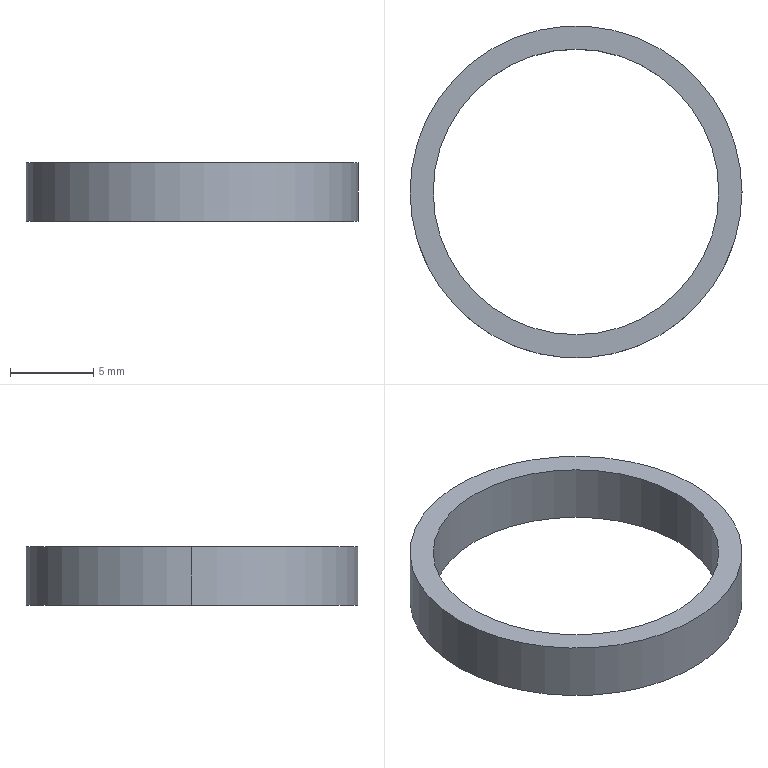Part | NX | features BREP 1 | 1 solid | 6 faces | box 20 x 20 x 3.5 mm | volume 286.325 mm3 | cylinder 4 | plane 2 | commonest cylinder face diameters 17.2 x2 20 x2
STEP:
#1=CARTESIAN_POINT('',(-8.6,0.,0.));
#2=VERTEX_POINT('',#1);
#3=CARTESIAN_POINT('',(8.6,0.,0.));
#4=VERTEX_POINT('',#3);
#5=CARTESIAN_POINT('',(0.,0.,0.));
#6=DIRECTION('',(0.,0.,1.));
#7=DIRECTION('',(1.,0.,0.));
#8=AXIS2_PLACEMENT_3D('',#5,#6,#7);
#9=CIRCLE('',#8,8.6);
#10=EDGE_CURVE('',#2,#4,#9,.T.);
#11=ORIENTED_EDGE('',*,*,#10,.F.);
#12=CARTESIAN_POINT('',(-8.6,0.,3.5));
#13=VERTEX_POINT('',#12);
#14=CARTESIAN_POINT('',(-8.6,0.,0.));
#15=DIRECTION('',(0.,0.,1.));
#16=VECTOR('',#15,1000.);
#17=LINE('',#14,#16);
#18=EDGE_CURVE('',#13,#2,#17,.F.);
#19=ORIENTED_EDGE('',*,*,#18,.F.);
#20=CARTESIAN_POINT('',(8.6,0.,3.5));
#21=VERTEX_POINT('',#20);
#22=CARTESIAN_POINT('',(0.,0.,3.5));
#23=DIRECTION('',(0.,0.,1.));
#24=DIRECTION('',(1.,0.,0.));
#25=AXIS2_PLACEMENT_3D('',#22,#23,#24);
#26=CIRCLE('',#25,8.6);
#27=EDGE_CURVE('',#13,#21,#26,.T.);
#28=ORIENTED_EDGE('',*,*,#27,.T.);
#29=CARTESIAN_POINT('',(8.6,0.,0.));
#30=DIRECTION('',(0.,0.,1.));
#31=VECTOR('',#30,1000.);
#32=LINE('',#29,#31);
#33=EDGE_CURVE('',#21,#4,#32,.F.);
#34=ORIENTED_EDGE('',*,*,#33,.T.);
#35=EDGE_LOOP('',(#11,#19,#28,#34));
#36=FACE_BOUND('',#35,.T.);
#37=CARTESIAN_POINT('',(0.,0.,0.));
#38=DIRECTION('',(0.,0.,1.));
#39=DIRECTION('',(1.,0.,0.));
#40=AXIS2_PLACEMENT_3D('',#37,#38,#39);
#41=CYLINDRICAL_SURFACE('',#40,8.6);
#42=ADVANCED_FACE('',(#36),#41,.F.);
#43=CARTESIAN_POINT('',(10.,0.,3.5));
#44=VERTEX_POINT('',#43);
#45=CARTESIAN_POINT('',(-10.,0.,3.5));
#46=VERTEX_POINT('',#45);
#47=CARTESIAN_POINT('',(0.,0.,3.5));
#48=DIRECTION('',(0.,0.,1.));
#49=DIRECTION('',(1.,0.,0.));
#50=AXIS2_PLACEMENT_3D('',#47,#48,#49);
#51=CIRCLE('',#50,10.);
#52=EDGE_CURVE('',#44,#46,#51,.T.);
#53=ORIENTED_EDGE('',*,*,#52,.F.);
#54=CARTESIAN_POINT('',(10.,0.,0.));
#55=VERTEX_POINT('',#54);
#56=CARTESIAN_POINT('',(10.,0.,3.5));
#57=DIRECTION('',(0.,0.,-1.));
#58=VECTOR('',#57,1000.);
#59=LINE('',#56,#58);
#60=EDGE_CURVE('',#44,#55,#59,.T.);
#61=ORIENTED_EDGE('',*,*,#60,.T.);
#62=CARTESIAN_POINT('',(-10.,0.,0.));
#63=VERTEX_POINT('',#62);
#64=CARTESIAN_POINT('',(0.,0.,0.));
#65=DIRECTION('',(0.,0.,1.));
#66=DIRECTION('',(1.,0.,0.));
#67=AXIS2_PLACEMENT_3D('',#64,#65,#66);
#68=CIRCLE('',#67,10.);
#69=EDGE_CURVE('',#55,#63,#68,.T.);
#70=ORIENTED_EDGE('',*,*,#69,.T.);
#71=CARTESIAN_POINT('',(-10.,0.,3.5));
#72=DIRECTION('',(0.,0.,-1.));
#73=VECTOR('',#72,1000.);
#74=LINE('',#71,#73);
#75=EDGE_CURVE('',#46,#63,#74,.T.);
#76=ORIENTED_EDGE('',*,*,#75,.F.);
#77=EDGE_LOOP('',(#53,#61,#70,#76));
#78=FACE_BOUND('',#77,.T.);
#79=CARTESIAN_POINT('',(0.,0.,3.5));
#80=DIRECTION('',(0.,0.,-1.));
#81=DIRECTION('',(-1.,0.,0.));
#82=AXIS2_PLACEMENT_3D('',#79,#80,#81);
#83=CYLINDRICAL_SURFACE('',#82,10.);
#84=ADVANCED_FACE('',(#78),#83,.T.);
#85=ORIENTED_EDGE('',*,*,#60,.F.);
#86=CARTESIAN_POINT('',(0.,0.,3.5));
#87=DIRECTION('',(0.,0.,1.));
#88=DIRECTION('',(1.,0.,0.));
#89=AXIS2_PLACEMENT_3D('',#86,#87,#88);
#90=CIRCLE('',#89,10.);
#91=EDGE_CURVE('',#46,#44,#90,.T.);
#92=ORIENTED_EDGE('',*,*,#91,.F.);
#93=ORIENTED_EDGE('',*,*,#75,.T.);
#94=CARTESIAN_POINT('',(0.,0.,0.));
#95=DIRECTION('',(0.,0.,1.));
#96=DIRECTION('',(1.,0.,0.));
#97=AXIS2_PLACEMENT_3D('',#94,#95,#96);
#98=CIRCLE('',#97,10.);
#99=EDGE_CURVE('',#63,#55,#98,.T.);
#100=ORIENTED_EDGE('',*,*,#99,.T.);
#101=EDGE_LOOP('',(#85,#92,#93,#100));
#102=FACE_BOUND('',#101,.T.);
#103=CARTESIAN_POINT('',(0.,0.,3.5));
#104=DIRECTION('',(0.,0.,-1.));
#105=DIRECTION('',(-1.,0.,0.));
#106=AXIS2_PLACEMENT_3D('',#103,#104,#105);
#107=CYLINDRICAL_SURFACE('',#106,10.);
#108=ADVANCED_FACE('',(#102),#107,.T.);
#109=ORIENTED_EDGE('',*,*,#91,.T.);
#110=ORIENTED_EDGE('',*,*,#52,.T.);
#111=EDGE_LOOP('',(#109,#110));
#112=FACE_BOUND('',#111,.T.);
#113=CARTESIAN_POINT('',(0.,0.,3.5));
#114=DIRECTION('',(0.,0.,1.));
#115=DIRECTION('',(1.,0.,0.));
#116=AXIS2_PLACEMENT_3D('',#113,#114,#115);
#117=CIRCLE('',#116,8.6);
#118=EDGE_CURVE('',#21,#13,#117,.T.);
#119=ORIENTED_EDGE('',*,*,#118,.F.);
#120=ORIENTED_EDGE('',*,*,#27,.F.);
#121=EDGE_LOOP('',(#119,#120));
#122=FACE_BOUND('',#121,.T.);
#123=CARTESIAN_POINT('',(0.,0.,3.5));
#124=DIRECTION('',(0.,0.,1.));
#125=DIRECTION('',(1.,0.,0.));
#126=AXIS2_PLACEMENT_3D('',#123,#124,#125);
#127=PLANE('',#126);
#128=ADVANCED_FACE('',(#112,#122),#127,.T.);
#129=ORIENTED_EDGE('',*,*,#99,.F.);
#130=ORIENTED_EDGE('',*,*,#69,.F.);
#131=EDGE_LOOP('',(#129,#130));
#132=FACE_BOUND('',#131,.T.);
#133=CARTESIAN_POINT('',(0.,0.,0.));
#134=DIRECTION('',(0.,0.,1.));
#135=DIRECTION('',(1.,0.,0.));
#136=AXIS2_PLACEMENT_3D('',#133,#134,#135);
#137=CIRCLE('',#136,8.6);
#138=EDGE_CURVE('',#4,#2,#137,.T.);
#139=ORIENTED_EDGE('',*,*,#138,.T.);
#140=ORIENTED_EDGE('',*,*,#10,.T.);
#141=EDGE_LOOP('',(#139,#140));
#142=FACE_BOUND('',#141,.T.);
#143=CARTESIAN_POINT('',(0.,0.,0.));
#144=DIRECTION('',(0.,0.,1.));
#145=DIRECTION('',(1.,0.,0.));
#146=AXIS2_PLACEMENT_3D('',#143,#144,#145);
#147=PLANE('',#146);
#148=ADVANCED_FACE('',(#132,#142),#147,.F.);
#149=ORIENTED_EDGE('',*,*,#18,.T.);
#150=ORIENTED_EDGE('',*,*,#138,.F.);
#151=ORIENTED_EDGE('',*,*,#33,.F.);
#152=ORIENTED_EDGE('',*,*,#118,.T.);
#153=EDGE_LOOP('',(#149,#150,#151,#152));
#154=FACE_BOUND('',#153,.T.);
#155=CARTESIAN_POINT('',(0.,0.,0.));
#156=DIRECTION('',(0.,0.,1.));
#157=DIRECTION('',(1.,0.,0.));
#158=AXIS2_PLACEMENT_3D('',#155,#156,#157);
#159=CYLINDRICAL_SURFACE('',#158,8.6);
#160=ADVANCED_FACE('',(#154),#159,.F.);
#161=CLOSED_SHELL('',(#42,#84,#108,#128,#148,#160));
#162=MANIFOLD_SOLID_BREP('',#161);
#163=(LENGTH_UNIT()NAMED_UNIT(*)SI_UNIT(.MILLI.,.METRE.));
#164=UNCERTAINTY_MEASURE_WITH_UNIT(LENGTH_MEASURE(0.00001),#163,'','');
#165=(NAMED_UNIT(*)PLANE_ANGLE_UNIT()SI_UNIT($,.RADIAN.));
#166=(NAMED_UNIT(*)SI_UNIT($,.STERADIAN.)SOLID_ANGLE_UNIT());
#167=(GEOMETRIC_REPRESENTATION_CONTEXT(3)GLOBAL_UNCERTAINTY_ASSIGNED_CONTEXT((#164))GLOBAL_UNIT_ASSIGNED_CONTEXT((#163,#165,#166))REPRESENTATION_CONTEXT('',''));
#168=ADVANCED_BREP_SHAPE_REPRESENTATION('',(#162),#167);